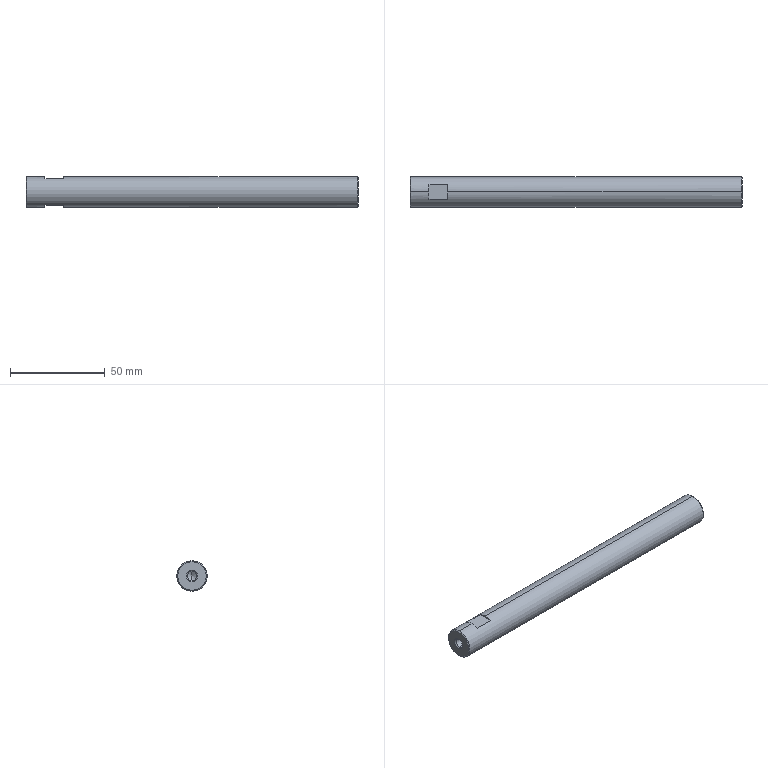Part | STEP file | sfjz16_175_m6_n6_sc10_2_03 | 1 solid | 26 faces | box 175 x 16 x 16 mm | volume 34378 mm3 | cone 12 | plane 8 | cylinder 6 | commonest cylinder face diameters 4.917 x4 16 x2